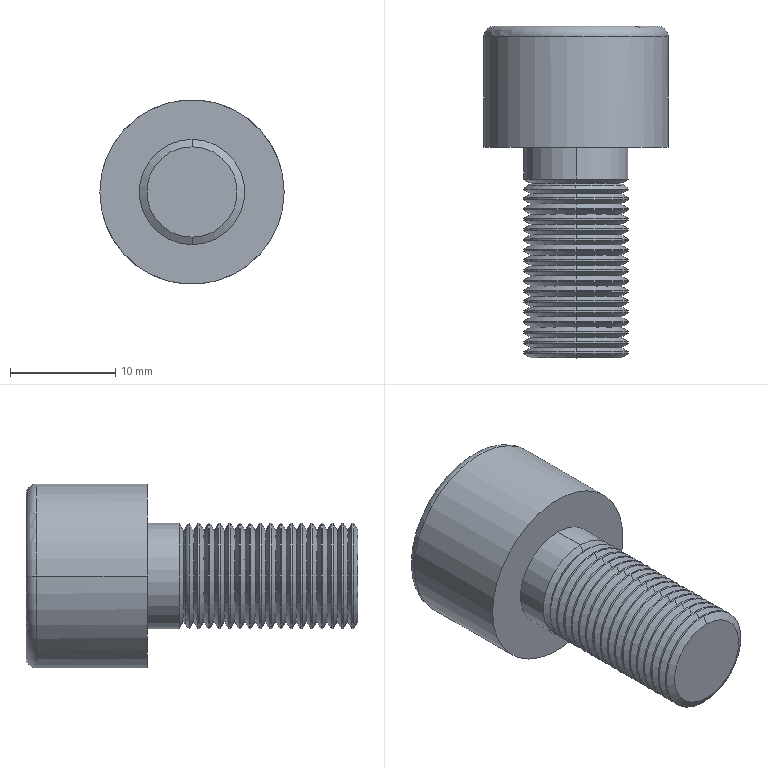Part | SolidWorks | features BaseBody 1 | 1 solid | 125 faces | box 17.5 x 31.5 x 17.5 mm | volume 3873 mm3 | cone 70 | cylinder 36 | plane 15 | torus 4 | commonest cylinder face diameters 10 x34 17.5 x2